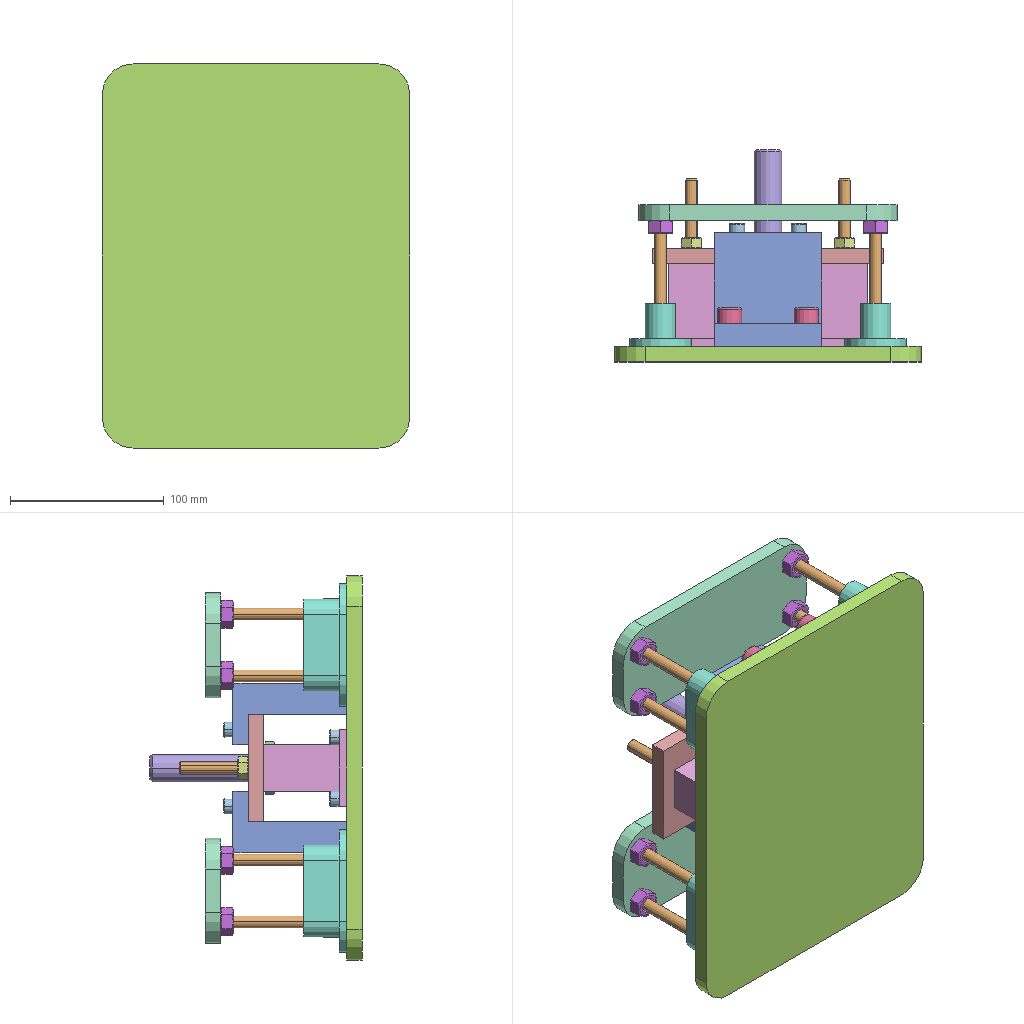Assembly | SolidWorks | 13 different items | 55 placed | box 200 x 138 x 250 mm
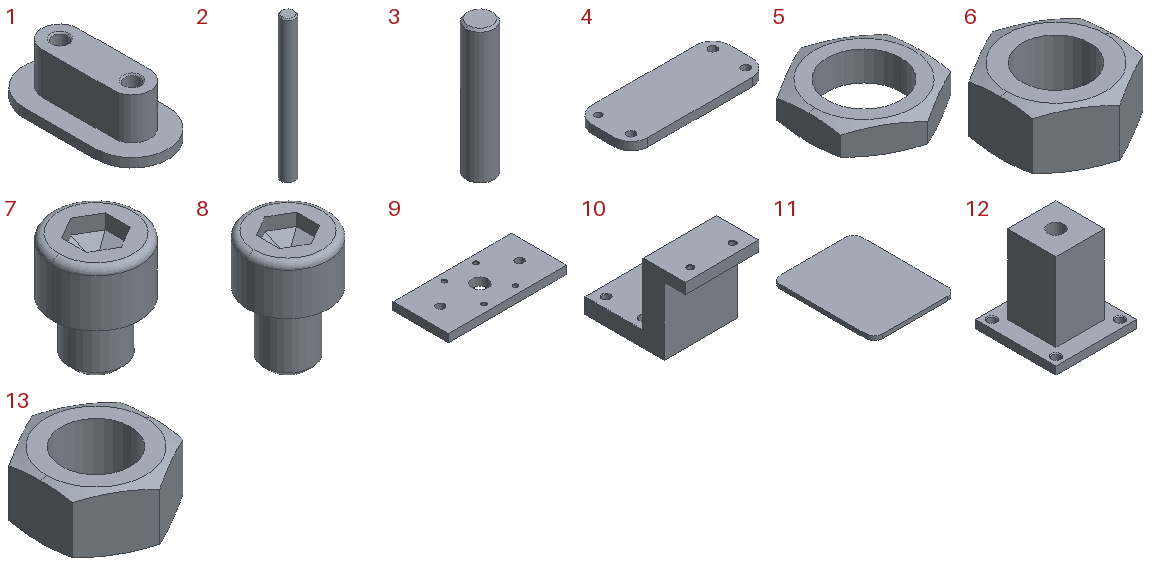Parts list (item | quantity | size | volume | features):
1 | x4 | 40 x 80 x 28 mm | 37305 mm3 | features Extrusion 1, HoleWzd 1, ICE 1
2 | x11 | 8 x 8 x 83 mm | 4167 mm3 | features Extrusion 1, StudWizard 1
3 | x1 | 18 x 18 x 86 mm | 21835 mm3 | features Extrusion 1, StudWizard 1
4 | x2 | 168 x 68.566 x 10 mm | 108898 mm3 | features Cut 1, Extrusion 1, Fillet 1
5 | x1 | 30 x 34.641 x 8 mm | 3531 mm3 | features Extrusion 1, ICE 1, MirrorPattern 1, RefAxis 1, RevCut 1
6 | x2 | 13 x 15.011 x 6.8 mm | 637.901 mm3 | features Extrusion 1, ICE 1, MirrorPattern 1, RefAxis 1, RevCut 1
7 | x8 | 16 x 16 x 20 mm | 2566 mm3 | features Chamfer 2, Fillet 2, ICE 2, Extrusion 1, RefAxis 1
8 | x12 | 10 x 10 x 14 mm | 644.591 mm3 | features Chamfer 2, Fillet 2, ICE 2, Extrusion 1, RefAxis 1
9 | x1 | 150 x 70 x 10 mm | 99493 mm3 | features Cut 2, Extrusion 1, HoleWzd 1
10 | x2 | 70 x 95 x 74 mm | 172756 mm3 | features HoleWzd 2, ICE 2, Extrusion 1
11 | x1 | 200 x 250 x 10 mm | 494356 mm3 | features HoleWzd 2, Extrusion 1, Fillet 1
12 | x2 | 50 x 50 x 54 mm | 53135 mm3 | features Cut 1, Extrusion 1, HoleWzd 1, ICE 1
13 | x8 | 16 x 18.475 x 8.4 mm | 1174 mm3 | features Extrusion 1, ICE 1, MirrorPattern 1, RefAxis 1, RevCut 1
Mates (type | each side: item.copy, entity, surface, feature):
InPlace | 9.1 plane | assembly plane
InPlace | 9.1 face plane Boss-Extrude 1 | 10.1 plane
InPlace | 10.1 face plane Boss-Extrude 1 | 11.1 plane
InPlace | 11.1 face plane Boss-Extrude 1 | 12.1 plane
InPlace | 11.1 face plane Boss-Extrude 1 | 1.1 plane
InPlace | 1.1 face plane Boss-Extrude 1 | 2.1 plane
Concentric | 1.1 face cylinder M10 Tapped Hole 1 | 2.2 face cylinder M8 MechanicalThread Unnamed1
Coincident | 2.1 face plane Boss-Extrude 1 | 2.2 face plane Boss-Extrude 1
InPlace | 9.1 face plane Boss-Extrude 1 | 3.1 plane
Coincident | 9.1 face plane Boss-Extrude 1 | assembly plane
Concentric | 3.1 face cylinder M18 MechanicalThread Unnamed1 | assembly axis
Coincident | 9.1 face plane Boss-Extrude 1 | 5.1 plane
Concentric | 3.1 face cylinder M18 MechanicalThread Unnamed1 | 5.1 axis
Coincident | 10.1 face plane Boss-Extrude 3 | 7.1 plane
Concentric | 10.1 face cylinder M8 Tapped Hole 1 | 7.1 axis
Coincident | 10.1 face plane Boss-Extrude 3 | 7.2 plane
Concentric | 10.1 face cylinder M8 Tapped Hole 1 | 7.2 axis
Coincident | 10.1 face plane Boss-Extrude 3 | 7.3 plane
Concentric | 10.1 face cylinder M8 Tapped Hole 1 | 7.3 axis
Coincident | 10.1 face plane Boss-Extrude 3 | 7.4 plane
Concentric | 10.1 face cylinder M8 Tapped Hole 1 | 7.4 axis
Coincident | 12.1 face plane Boss-Extrude 2 | 8.1 plane
Concentric | 12.1 face cylinder M6 Tapped Hole 1 | 8.1 axis
Coincident | 12.1 face plane Boss-Extrude 2 | 8.2 plane
Concentric | 12.1 face cylinder M6 Tapped Hole 1 | 8.2 axis
Coincident | 12.1 face plane Boss-Extrude 2 | 8.3 plane
Concentric | 12.1 face cylinder M6 Tapped Hole 1 | 8.3 axis
Coincident | 12.1 face plane Boss-Extrude 2 | 8.4 plane
Concentric | 12.1 face cylinder M6 Tapped Hole 1 | 8.4 axis
Coincident | 10.1 face plane Boss-Extrude 1 | 8.5 plane
Concentric | 10.1 face cylinder M6 Tapped Hole 1 | 8.5 axis
Coincident | 10.1 face plane Boss-Extrude 1 | 8.6 plane
Concentric | 10.1 face cylinder M6 Tapped Hole 1 | 8.6 axis
Concentric | 9.1 face cylinder Cut-Extrude 2 | 2.3 face cylinder M8 MechanicalThread Unnamed1
DistanceDim | 9.1 face plane Boss-Extrude 1 | 2.3 face plane Boss-Extrude 1
Concentric | 9.1 face cylinder Cut-Extrude 2 | 2.4 face cylinder M8 MechanicalThread Unnamed1
Coincident | 2.3 face plane Boss-Extrude 1 | 2.4 face plane Boss-Extrude 1
Coincident | 9.1 face plane Boss-Extrude 1 | 6.1 plane
Concentric | 2.4 face cylinder M8 MechanicalThread Unnamed1 | 6.1 axis
InPlace | 2.1 face plane Boss-Extrude 1 | 4.1 plane
Coincident | 4.1 face plane Boss-Extrude 1 | 13.1 plane
Concentric | 2.1 face cylinder M8 MechanicalThread Unnamed1 | 13.1 axis
Coincident | 4.1 face plane Boss-Extrude 1 | 13.2 plane
Concentric | 2.5 face cylinder M8 MechanicalThread Unnamed1 | 13.2 axis
Coincident | 4.1 face plane Boss-Extrude 1 | 13.3 plane
Concentric | 2.6 face cylinder M8 MechanicalThread Unnamed1 | 13.3 axis
Coincident | 4.1 face plane Boss-Extrude 1 | 13.4 plane
Concentric | 2.2 face cylinder M8 MechanicalThread Unnamed1 | 13.4 axis